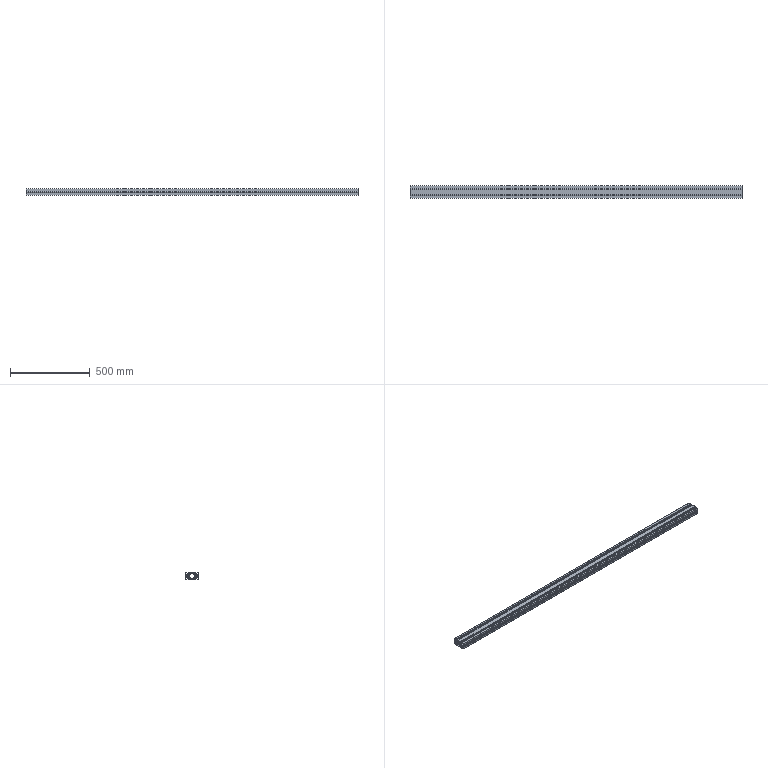Part | STEP file | Aluminium profile frame 2_Default<Machined> | 1 solid | 124 faces | box 2080 x 80 x 40 mm | volume 1541424 mm3 | plane 110 | cylinder 14 | commonest cylinder face diameters 9.6 x9 0.6 x2 6.6 x2 13.3 x1